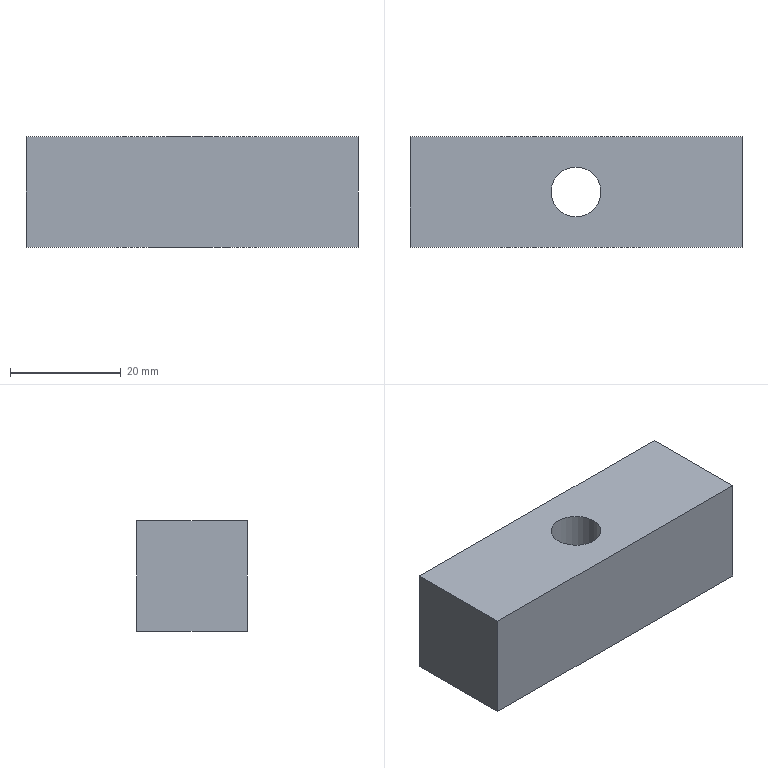Part | NX | features solid 2 | 1 solid | 9 faces | box 60 x 20 x 20 mm | volume 22095 mm3 | plane 7 | cylinder 2 | commonest cylinder face diameters 9 x1 14 x1
STEP:
#1=CARTESIAN_POINT('',(1555.,475.,42.));
#2=VERTEX_POINT('',#1);
#3=CARTESIAN_POINT('',(1555.,475.,22.));
#4=VERTEX_POINT('',#3);
#5=CARTESIAN_POINT('',(1555.,475.,42.));
#6=DIRECTION('',(0.,0.,1.));
#7=VECTOR('',#6,1000.);
#8=LINE('',#5,#7);
#9=EDGE_CURVE('',#2,#4,#8,.F.);
#10=ORIENTED_EDGE('',*,*,#9,.F.);
#11=CARTESIAN_POINT('',(1615.,475.,42.));
#12=VERTEX_POINT('',#11);
#13=CARTESIAN_POINT('',(1549.847,475.,42.));
#14=DIRECTION('',(-1.,0.,0.));
#15=VECTOR('',#14,1000.);
#16=LINE('',#13,#15);
#17=EDGE_CURVE('',#2,#12,#16,.F.);
#18=ORIENTED_EDGE('',*,*,#17,.T.);
#19=CARTESIAN_POINT('',(1615.,475.,22.));
#20=VERTEX_POINT('',#19);
#21=CARTESIAN_POINT('',(1615.,475.,42.));
#22=DIRECTION('',(0.,0.,-1.));
#23=VECTOR('',#22,1000.);
#24=LINE('',#21,#23);
#25=EDGE_CURVE('',#12,#20,#24,.T.);
#26=ORIENTED_EDGE('',*,*,#25,.T.);
#27=CARTESIAN_POINT('',(1549.847,475.,22.));
#28=DIRECTION('',(-1.,0.,0.));
#29=VECTOR('',#28,1000.);
#30=LINE('',#27,#29);
#31=EDGE_CURVE('',#4,#20,#30,.F.);
#32=ORIENTED_EDGE('',*,*,#31,.F.);
#33=EDGE_LOOP('',(#10,#18,#26,#32));
#34=FACE_BOUND('',#33,.T.);
#35=CARTESIAN_POINT('',(1549.847,475.,42.));
#36=DIRECTION('',(0.,1.,0.));
#37=DIRECTION('',(1.,0.,0.));
#38=AXIS2_PLACEMENT_3D('',#35,#36,#37);
#39=PLANE('',#38);
#40=ADVANCED_FACE('',(#34),#39,.T.);
#41=ORIENTED_EDGE('',*,*,#25,.F.);
#42=CARTESIAN_POINT('',(1615.,455.,42.));
#43=VERTEX_POINT('',#42);
#44=CARTESIAN_POINT('',(1615.,477.5,42.));
#45=DIRECTION('',(0.,1.,0.));
#46=VECTOR('',#45,1000.);
#47=LINE('',#44,#46);
#48=EDGE_CURVE('',#12,#43,#47,.F.);
#49=ORIENTED_EDGE('',*,*,#48,.T.);
#50=CARTESIAN_POINT('',(1615.,455.,22.));
#51=VERTEX_POINT('',#50);
#52=CARTESIAN_POINT('',(1615.,455.,42.));
#53=DIRECTION('',(0.,0.,1.));
#54=VECTOR('',#53,1000.);
#55=LINE('',#52,#54);
#56=EDGE_CURVE('',#43,#51,#55,.F.);
#57=ORIENTED_EDGE('',*,*,#56,.T.);
#58=CARTESIAN_POINT('',(1615.,477.5,22.));
#59=DIRECTION('',(0.,1.,0.));
#60=VECTOR('',#59,1000.);
#61=LINE('',#58,#60);
#62=EDGE_CURVE('',#20,#51,#61,.F.);
#63=ORIENTED_EDGE('',*,*,#62,.F.);
#64=EDGE_LOOP('',(#41,#49,#57,#63));
#65=FACE_BOUND('',#64,.T.);
#66=CARTESIAN_POINT('',(1615.,477.5,42.));
#67=DIRECTION('',(1.,0.,0.));
#68=DIRECTION('',(0.,-1.,0.));
#69=AXIS2_PLACEMENT_3D('',#66,#67,#68);
#70=PLANE('',#69);
#71=ADVANCED_FACE('',(#65),#70,.T.);
#72=ORIENTED_EDGE('',*,*,#56,.F.);
#73=CARTESIAN_POINT('',(1555.,455.,42.));
#74=VERTEX_POINT('',#73);
#75=CARTESIAN_POINT('',(1549.847,455.,42.));
#76=DIRECTION('',(1.,0.,0.));
#77=VECTOR('',#76,1000.);
#78=LINE('',#75,#77);
#79=EDGE_CURVE('',#74,#43,#78,.T.);
#80=ORIENTED_EDGE('',*,*,#79,.F.);
#81=CARTESIAN_POINT('',(1555.,455.,22.));
#82=VERTEX_POINT('',#81);
#83=CARTESIAN_POINT('',(1555.,455.,42.));
#84=DIRECTION('',(0.,0.,-1.));
#85=VECTOR('',#84,1000.);
#86=LINE('',#83,#85);
#87=EDGE_CURVE('',#74,#82,#86,.T.);
#88=ORIENTED_EDGE('',*,*,#87,.T.);
#89=CARTESIAN_POINT('',(1549.847,455.,22.));
#90=DIRECTION('',(1.,0.,0.));
#91=VECTOR('',#90,1000.);
#92=LINE('',#89,#91);
#93=EDGE_CURVE('',#82,#51,#92,.T.);
#94=ORIENTED_EDGE('',*,*,#93,.T.);
#95=EDGE_LOOP('',(#72,#80,#88,#94));
#96=FACE_BOUND('',#95,.T.);
#97=CARTESIAN_POINT('',(1549.847,455.,42.));
#98=DIRECTION('',(0.,1.,0.));
#99=DIRECTION('',(1.,0.,0.));
#100=AXIS2_PLACEMENT_3D('',#97,#98,#99);
#101=PLANE('',#100);
#102=ADVANCED_FACE('',(#96),#101,.F.);
#103=CARTESIAN_POINT('',(1555.,477.5,42.));
#104=DIRECTION('',(0.,-1.,0.));
#105=VECTOR('',#104,1000.);
#106=LINE('',#103,#105);
#107=EDGE_CURVE('',#2,#74,#106,.T.);
#108=ORIENTED_EDGE('',*,*,#107,.F.);
#109=ORIENTED_EDGE('',*,*,#9,.T.);
#110=CARTESIAN_POINT('',(1555.,477.5,22.));
#111=DIRECTION('',(0.,-1.,0.));
#112=VECTOR('',#111,1000.);
#113=LINE('',#110,#112);
#114=EDGE_CURVE('',#4,#82,#113,.T.);
#115=ORIENTED_EDGE('',*,*,#114,.T.);
#116=ORIENTED_EDGE('',*,*,#87,.F.);
#117=EDGE_LOOP('',(#108,#109,#115,#116));
#118=FACE_BOUND('',#117,.T.);
#119=CARTESIAN_POINT('',(1555.,477.5,42.));
#120=DIRECTION('',(1.,0.,0.));
#121=DIRECTION('',(0.,-1.,0.));
#122=AXIS2_PLACEMENT_3D('',#119,#120,#121);
#123=PLANE('',#122);
#124=ADVANCED_FACE('',(#118),#123,.F.);
#125=CARTESIAN_POINT('',(1578.,465.,22.));
#126=VERTEX_POINT('',#125);
#127=CARTESIAN_POINT('',(1585.,465.,22.));
#128=DIRECTION('',(0.,0.,-1.));
#129=DIRECTION('',(-1.,0.,0.));
#130=AXIS2_PLACEMENT_3D('',#127,#128,#129);
#131=CIRCLE('',#130,7.);
#132=EDGE_CURVE('',#126,#126,#131,.T.);
#133=ORIENTED_EDGE('',*,*,#132,.F.);
#134=EDGE_LOOP('',(#133));
#135=FACE_BOUND('',#134,.T.);
#136=ORIENTED_EDGE('',*,*,#93,.F.);
#137=ORIENTED_EDGE('',*,*,#114,.F.);
#138=ORIENTED_EDGE('',*,*,#31,.T.);
#139=ORIENTED_EDGE('',*,*,#62,.T.);
#140=EDGE_LOOP('',(#136,#137,#138,#139));
#141=FACE_BOUND('',#140,.T.);
#142=CARTESIAN_POINT('',(1549.847,477.5,22.));
#143=DIRECTION('',(0.,0.,1.));
#144=DIRECTION('',(1.,0.,0.));
#145=AXIS2_PLACEMENT_3D('',#142,#143,#144);
#146=PLANE('',#145);
#147=ADVANCED_FACE('',(#135,#141),#146,.F.);
#148=CARTESIAN_POINT('',(1580.5,465.,42.));
#149=VERTEX_POINT('',#148);
#150=CARTESIAN_POINT('',(1585.,465.,42.));
#151=DIRECTION('',(0.,0.,-1.));
#152=DIRECTION('',(-1.,0.,0.));
#153=AXIS2_PLACEMENT_3D('',#150,#151,#152);
#154=CIRCLE('',#153,4.5);
#155=EDGE_CURVE('',#149,#149,#154,.T.);
#156=ORIENTED_EDGE('',*,*,#155,.T.);
#157=EDGE_LOOP('',(#156));
#158=FACE_BOUND('',#157,.T.);
#159=ORIENTED_EDGE('',*,*,#79,.T.);
#160=ORIENTED_EDGE('',*,*,#48,.F.);
#161=ORIENTED_EDGE('',*,*,#17,.F.);
#162=ORIENTED_EDGE('',*,*,#107,.T.);
#163=EDGE_LOOP('',(#159,#160,#161,#162));
#164=FACE_BOUND('',#163,.T.);
#165=CARTESIAN_POINT('',(1549.847,477.5,42.));
#166=DIRECTION('',(0.,0.,1.));
#167=DIRECTION('',(1.,0.,0.));
#168=AXIS2_PLACEMENT_3D('',#165,#166,#167);
#169=PLANE('',#168);
#170=ADVANCED_FACE('',(#158,#164),#169,.T.);
#171=ORIENTED_EDGE('',*,*,#155,.F.);
#172=EDGE_LOOP('',(#171));
#173=FACE_BOUND('',#172,.T.);
#174=CARTESIAN_POINT('',(1580.5,465.,29.));
#175=VERTEX_POINT('',#174);
#176=CARTESIAN_POINT('',(1585.,465.,29.));
#177=DIRECTION('',(0.,0.,-1.));
#178=DIRECTION('',(-1.,0.,0.));
#179=AXIS2_PLACEMENT_3D('',#176,#177,#178);
#180=CIRCLE('',#179,4.5);
#181=EDGE_CURVE('',#175,#175,#180,.T.);
#182=ORIENTED_EDGE('',*,*,#181,.T.);
#183=EDGE_LOOP('',(#182));
#184=FACE_BOUND('',#183,.T.);
#185=CARTESIAN_POINT('',(1585.,465.,67.));
#186=DIRECTION('',(0.,0.,1.));
#187=DIRECTION('',(1.,0.,0.));
#188=AXIS2_PLACEMENT_3D('',#185,#186,#187);
#189=CYLINDRICAL_SURFACE('',#188,4.5);
#190=ADVANCED_FACE('',(#173,#184),#189,.F.);
#191=ORIENTED_EDGE('',*,*,#181,.F.);
#192=EDGE_LOOP('',(#191));
#193=FACE_BOUND('',#192,.T.);
#194=CARTESIAN_POINT('',(1578.,465.,29.));
#195=VERTEX_POINT('',#194);
#196=CARTESIAN_POINT('',(1585.,465.,29.));
#197=DIRECTION('',(0.,0.,-1.));
#198=DIRECTION('',(-1.,0.,0.));
#199=AXIS2_PLACEMENT_3D('',#196,#197,#198);
#200=CIRCLE('',#199,7.);
#201=EDGE_CURVE('',#195,#195,#200,.T.);
#202=ORIENTED_EDGE('',*,*,#201,.T.);
#203=EDGE_LOOP('',(#202));
#204=FACE_BOUND('',#203,.T.);
#205=CARTESIAN_POINT('',(1585.,465.,29.));
#206=DIRECTION('',(0.,0.,1.));
#207=DIRECTION('',(1.,0.,0.));
#208=AXIS2_PLACEMENT_3D('',#205,#206,#207);
#209=PLANE('',#208);
#210=ADVANCED_FACE('',(#193,#204),#209,.F.);
#211=ORIENTED_EDGE('',*,*,#201,.F.);
#212=EDGE_LOOP('',(#211));
#213=FACE_BOUND('',#212,.T.);
#214=ORIENTED_EDGE('',*,*,#132,.T.);
#215=EDGE_LOOP('',(#214));
#216=FACE_BOUND('',#215,.T.);
#217=CARTESIAN_POINT('',(1585.,465.,17.));
#218=DIRECTION('',(0.,0.,1.));
#219=DIRECTION('',(1.,0.,0.));
#220=AXIS2_PLACEMENT_3D('',#217,#218,#219);
#221=CYLINDRICAL_SURFACE('',#220,7.);
#222=ADVANCED_FACE('',(#213,#216),#221,.F.);
#223=CLOSED_SHELL('',(#40,#71,#102,#124,#147,#170,#190,#210,#222));
#224=MANIFOLD_SOLID_BREP('',#223);
#225=(LENGTH_UNIT()NAMED_UNIT(*)SI_UNIT(.MILLI.,.METRE.));
#226=UNCERTAINTY_MEASURE_WITH_UNIT(LENGTH_MEASURE(0.00001),#225,'','');
#227=(NAMED_UNIT(*)PLANE_ANGLE_UNIT()SI_UNIT($,.RADIAN.));
#228=(NAMED_UNIT(*)SI_UNIT($,.STERADIAN.)SOLID_ANGLE_UNIT());
#229=(GEOMETRIC_REPRESENTATION_CONTEXT(3)GLOBAL_UNCERTAINTY_ASSIGNED_CONTEXT((#226))GLOBAL_UNIT_ASSIGNED_CONTEXT((#225,#227,#228))REPRESENTATION_CONTEXT('',''));
#230=ADVANCED_BREP_SHAPE_REPRESENTATION('',(#224),#229);